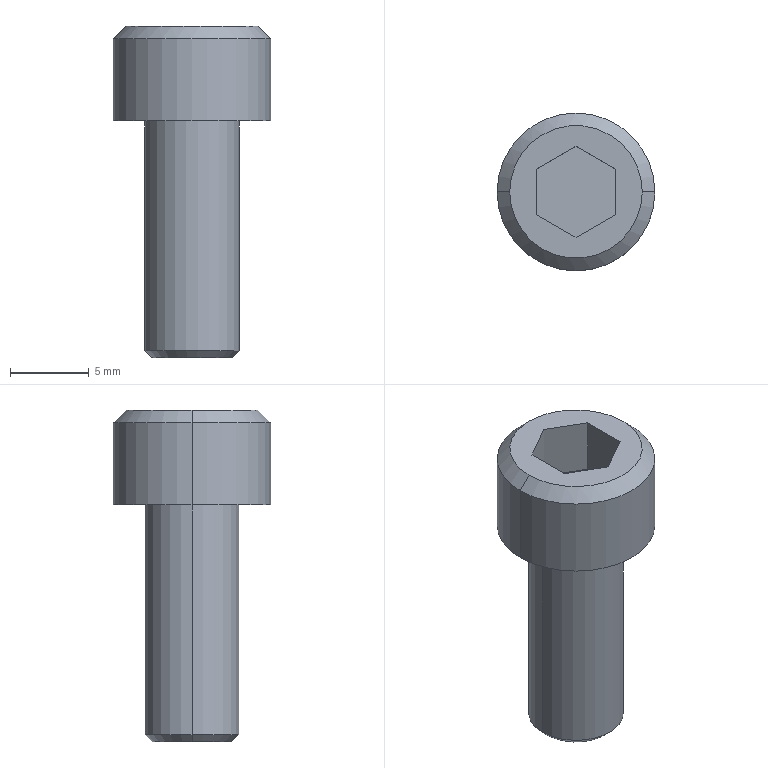Part | Creo | 1 solid | 18 faces | box 10 x 10 x 21 mm | volume 806.082 mm3 | plane 10 | cylinder 4 | cone 4 | commonest cylinder face diameters 6 x2 10 x2
STEP:
#1=CARTESIAN_POINT('',(-255.,152.592,-6.5));
#2=VERTEX_POINT('',#1);
#3=CARTESIAN_POINT('',(-265.,152.592,-6.5));
#4=VERTEX_POINT('',#3);
#5=CARTESIAN_POINT('',(-260.,152.592,-6.5));
#6=DIRECTION('',(0.,0.,-1.));
#7=DIRECTION('',(1.,0.,0.));
#8=AXIS2_PLACEMENT_3D('',#5,#6,#7);
#9=CIRCLE('',#8,5.);
#10=EDGE_CURVE('',#2,#4,#9,.T.);
#11=ORIENTED_EDGE('',*,*,#10,.F.);
#12=CARTESIAN_POINT('',(-260.,152.592,-6.5));
#13=DIRECTION('',(0.,0.,-1.));
#14=DIRECTION('',(-1.,0.,0.));
#15=AXIS2_PLACEMENT_3D('',#12,#13,#14);
#16=CIRCLE('',#15,5.);
#17=EDGE_CURVE('',#4,#2,#16,.T.);
#18=ORIENTED_EDGE('',*,*,#17,.F.);
#19=EDGE_LOOP('',(#11,#18));
#20=FACE_OUTER_BOUND('',#19,.F.);
#21=CARTESIAN_POINT('',(-263.,152.592,-6.5));
#22=VERTEX_POINT('',#21);
#23=CARTESIAN_POINT('',(-257.,152.592,-6.5));
#24=VERTEX_POINT('',#23);
#25=CARTESIAN_POINT('',(-260.,152.592,-6.5));
#26=DIRECTION('',(0.,0.,1.));
#27=DIRECTION('',(-1.,0.,0.));
#28=AXIS2_PLACEMENT_3D('',#25,#26,#27);
#29=CIRCLE('',#28,3.);
#30=EDGE_CURVE('',#22,#24,#29,.T.);
#31=ORIENTED_EDGE('',*,*,#30,.F.);
#32=CARTESIAN_POINT('',(-260.,152.592,-6.5));
#33=DIRECTION('',(0.,0.,1.));
#34=DIRECTION('',(1.,0.,0.));
#35=AXIS2_PLACEMENT_3D('',#32,#33,#34);
#36=CIRCLE('',#35,3.);
#37=EDGE_CURVE('',#24,#22,#36,.T.);
#38=ORIENTED_EDGE('',*,*,#37,.F.);
#39=EDGE_LOOP('',(#31,#38));
#40=FACE_BOUND('',#39,.F.);
#41=CARTESIAN_POINT('',(-260.,152.592,-6.5));
#42=DIRECTION('',(0.,0.,-1.));
#43=DIRECTION('',(-1.,0.,0.));
#44=AXIS2_PLACEMENT_3D('',#41,#42,#43);
#45=PLANE('',#44);
#46=ADVANCED_FACE('',(#20,#40),#45,.T.);
#47=CARTESIAN_POINT('',(-257.,152.592,-21.05));
#48=VERTEX_POINT('',#47);
#49=CARTESIAN_POINT('',(-263.,152.592,-21.05));
#50=VERTEX_POINT('',#49);
#51=CARTESIAN_POINT('',(-260.,152.592,-21.05));
#52=DIRECTION('',(0.,0.,-1.));
#53=DIRECTION('',(1.,0.,0.));
#54=AXIS2_PLACEMENT_3D('',#51,#52,#53);
#55=CIRCLE('',#54,3.);
#56=EDGE_CURVE('',#48,#50,#55,.T.);
#57=ORIENTED_EDGE('',*,*,#56,.T.);
#58=CARTESIAN_POINT('',(-263.,152.592,-6.5));
#59=DIRECTION('',(0.,0.,-1.));
#60=VECTOR('',#59,14.55);
#61=LINE('',#58,#60);
#62=EDGE_CURVE('',#22,#50,#61,.T.);
#63=ORIENTED_EDGE('',*,*,#62,.F.);
#64=ORIENTED_EDGE('',*,*,#30,.T.);
#65=CARTESIAN_POINT('',(-257.,152.592,-6.5));
#66=DIRECTION('',(0.,0.,-1.));
#67=VECTOR('',#66,14.55);
#68=LINE('',#65,#67);
#69=EDGE_CURVE('',#24,#48,#68,.T.);
#70=ORIENTED_EDGE('',*,*,#69,.T.);
#71=EDGE_LOOP('',(#57,#63,#64,#70));
#72=FACE_OUTER_BOUND('',#71,.F.);
#73=CARTESIAN_POINT('',(-260.,152.592,0.5));
#74=DIRECTION('',(0.,0.,-1.));
#75=DIRECTION('',(-1.,0.,0.));
#76=AXIS2_PLACEMENT_3D('',#73,#74,#75);
#77=CYLINDRICAL_SURFACE('',#76,3.);
#78=ADVANCED_FACE('',(#72),#77,.T.);
#79=CARTESIAN_POINT('',(-257.45,152.592,-21.5));
#80=VERTEX_POINT('',#79);
#81=CARTESIAN_POINT('',(-262.55,152.592,-21.5));
#82=VERTEX_POINT('',#81);
#83=CARTESIAN_POINT('',(-260.,152.592,-21.5));
#84=DIRECTION('',(0.,0.,-1.));
#85=DIRECTION('',(1.,0.,0.));
#86=AXIS2_PLACEMENT_3D('',#83,#84,#85);
#87=CIRCLE('',#86,2.55);
#88=EDGE_CURVE('',#80,#82,#87,.T.);
#89=ORIENTED_EDGE('',*,*,#88,.T.);
#90=CARTESIAN_POINT('',(-262.55,152.592,-21.5));
#91=DIRECTION('',(-0.7071,0.,0.7071));
#92=VECTOR('',#91,0.6364);
#93=LINE('',#90,#92);
#94=EDGE_CURVE('',#82,#50,#93,.T.);
#95=ORIENTED_EDGE('',*,*,#94,.T.);
#96=ORIENTED_EDGE('',*,*,#56,.F.);
#97=CARTESIAN_POINT('',(-257.45,152.592,-21.5));
#98=DIRECTION('',(0.7071,0.,0.7071));
#99=VECTOR('',#98,0.6364);
#100=LINE('',#97,#99);
#101=EDGE_CURVE('',#80,#48,#100,.T.);
#102=ORIENTED_EDGE('',*,*,#101,.F.);
#103=EDGE_LOOP('',(#89,#95,#96,#102));
#104=FACE_OUTER_BOUND('',#103,.F.);
#105=CARTESIAN_POINT('',(-260.,152.592,-21.275));
#106=DIRECTION('',(0.,0.,1.));
#107=DIRECTION('',(1.,0.,0.));
#108=AXIS2_PLACEMENT_3D('',#105,#106,#107);
#109=CONICAL_SURFACE('',#108,2.775,45.);
#110=ADVANCED_FACE('',(#104),#109,.T.);
#111=CARTESIAN_POINT('',(-260.,152.592,-21.5));
#112=DIRECTION('',(0.,0.,-1.));
#113=DIRECTION('',(-1.,0.,0.));
#114=AXIS2_PLACEMENT_3D('',#111,#112,#113);
#115=CIRCLE('',#114,2.55);
#116=EDGE_CURVE('',#82,#80,#115,.T.);
#117=ORIENTED_EDGE('',*,*,#116,.F.);
#118=ORIENTED_EDGE('',*,*,#88,.F.);
#119=EDGE_LOOP('',(#117,#118));
#120=FACE_OUTER_BOUND('',#119,.F.);
#121=CARTESIAN_POINT('',(-260.,152.592,-21.5));
#122=DIRECTION('',(0.,0.,-1.));
#123=DIRECTION('',(-1.,0.,0.));
#124=AXIS2_PLACEMENT_3D('',#121,#122,#123);
#125=PLANE('',#124);
#126=ADVANCED_FACE('',(#120),#125,.T.);
#127=ORIENTED_EDGE('',*,*,#116,.T.);
#128=ORIENTED_EDGE('',*,*,#101,.T.);
#129=CARTESIAN_POINT('',(-260.,152.592,-21.05));
#130=DIRECTION('',(0.,0.,-1.));
#131=DIRECTION('',(-1.,0.,0.));
#132=AXIS2_PLACEMENT_3D('',#129,#130,#131);
#133=CIRCLE('',#132,3.);
#134=EDGE_CURVE('',#50,#48,#133,.T.);
#135=ORIENTED_EDGE('',*,*,#134,.F.);
#136=ORIENTED_EDGE('',*,*,#94,.F.);
#137=EDGE_LOOP('',(#127,#128,#135,#136));
#138=FACE_OUTER_BOUND('',#137,.F.);
#139=CARTESIAN_POINT('',(-260.,152.592,-21.275));
#140=DIRECTION('',(0.,0.,1.));
#141=DIRECTION('',(1.,0.,0.));
#142=AXIS2_PLACEMENT_3D('',#139,#140,#141);
#143=CONICAL_SURFACE('',#142,2.775,45.);
#144=ADVANCED_FACE('',(#138),#143,.T.);
#145=ORIENTED_EDGE('',*,*,#134,.T.);
#146=ORIENTED_EDGE('',*,*,#69,.F.);
#147=ORIENTED_EDGE('',*,*,#37,.T.);
#148=ORIENTED_EDGE('',*,*,#62,.T.);
#149=EDGE_LOOP('',(#145,#146,#147,#148));
#150=FACE_OUTER_BOUND('',#149,.F.);
#151=CARTESIAN_POINT('',(-260.,152.592,0.5));
#152=DIRECTION('',(0.,0.,-1.));
#153=DIRECTION('',(-1.,0.,0.));
#154=AXIS2_PLACEMENT_3D('',#151,#152,#153);
#155=CYLINDRICAL_SURFACE('',#154,3.);
#156=ADVANCED_FACE('',(#150),#155,.T.);
#157=CARTESIAN_POINT('',(-265.,152.592,-1.3));
#158=VERTEX_POINT('',#157);
#159=CARTESIAN_POINT('',(-255.,152.592,-1.3));
#160=VERTEX_POINT('',#159);
#161=CARTESIAN_POINT('',(-260.,152.592,-1.3));
#162=DIRECTION('',(0.,0.,1.));
#163=DIRECTION('',(-1.,0.,0.));
#164=AXIS2_PLACEMENT_3D('',#161,#162,#163);
#165=CIRCLE('',#164,5.);
#166=EDGE_CURVE('',#158,#160,#165,.T.);
#167=ORIENTED_EDGE('',*,*,#166,.T.);
#168=CARTESIAN_POINT('',(-255.,152.592,-1.3));
#169=DIRECTION('',(0.,0.,-1.));
#170=VECTOR('',#169,5.2);
#171=LINE('',#168,#170);
#172=EDGE_CURVE('',#160,#2,#171,.T.);
#173=ORIENTED_EDGE('',*,*,#172,.T.);
#174=ORIENTED_EDGE('',*,*,#10,.T.);
#175=CARTESIAN_POINT('',(-265.,152.592,-1.3));
#176=DIRECTION('',(0.,0.,-1.));
#177=VECTOR('',#176,5.2);
#178=LINE('',#175,#177);
#179=EDGE_CURVE('',#158,#4,#178,.T.);
#180=ORIENTED_EDGE('',*,*,#179,.F.);
#181=EDGE_LOOP('',(#167,#173,#174,#180));
#182=FACE_OUTER_BOUND('',#181,.F.);
#183=CARTESIAN_POINT('',(-260.,152.592,0.5));
#184=DIRECTION('',(0.,0.,-1.));
#185=DIRECTION('',(-1.,0.,0.));
#186=AXIS2_PLACEMENT_3D('',#183,#184,#185);
#187=CYLINDRICAL_SURFACE('',#186,5.);
#188=ADVANCED_FACE('',(#182),#187,.T.);
#189=CARTESIAN_POINT('',(-264.2,152.592,-0.5));
#190=VERTEX_POINT('',#189);
#191=CARTESIAN_POINT('',(-255.8,152.592,-0.5));
#192=VERTEX_POINT('',#191);
#193=CARTESIAN_POINT('',(-260.,152.592,-0.5));
#194=DIRECTION('',(0.,0.,1.));
#195=DIRECTION('',(-1.,0.,0.));
#196=AXIS2_PLACEMENT_3D('',#193,#194,#195);
#197=CIRCLE('',#196,4.2);
#198=EDGE_CURVE('',#190,#192,#197,.T.);
#199=ORIENTED_EDGE('',*,*,#198,.T.);
#200=CARTESIAN_POINT('',(-255.8,152.592,-0.5));
#201=DIRECTION('',(0.7071,0.,-0.7071));
#202=VECTOR('',#201,1.131);
#203=LINE('',#200,#202);
#204=EDGE_CURVE('',#192,#160,#203,.T.);
#205=ORIENTED_EDGE('',*,*,#204,.T.);
#206=ORIENTED_EDGE('',*,*,#166,.F.);
#207=CARTESIAN_POINT('',(-264.2,152.592,-0.5));
#208=DIRECTION('',(-0.7071,0.,-0.7071));
#209=VECTOR('',#208,1.131);
#210=LINE('',#207,#209);
#211=EDGE_CURVE('',#190,#158,#210,.T.);
#212=ORIENTED_EDGE('',*,*,#211,.F.);
#213=EDGE_LOOP('',(#199,#205,#206,#212));
#214=FACE_OUTER_BOUND('',#213,.F.);
#215=CARTESIAN_POINT('',(-260.,152.592,-0.9));
#216=DIRECTION('',(0.,0.,-1.));
#217=DIRECTION('',(-1.,0.,0.));
#218=AXIS2_PLACEMENT_3D('',#215,#216,#217);
#219=CONICAL_SURFACE('',#218,4.6,45.);
#220=ADVANCED_FACE('',(#214),#219,.T.);
#221=ORIENTED_EDGE('',*,*,#198,.F.);
#222=CARTESIAN_POINT('',(-260.,152.592,-0.5));
#223=DIRECTION('',(0.,0.,1.));
#224=DIRECTION('',(1.,0.,0.));
#225=AXIS2_PLACEMENT_3D('',#222,#223,#224);
#226=CIRCLE('',#225,4.2);
#227=EDGE_CURVE('',#192,#190,#226,.T.);
#228=ORIENTED_EDGE('',*,*,#227,.F.);
#229=EDGE_LOOP('',(#221,#228));
#230=FACE_OUTER_BOUND('',#229,.F.);
#231=CARTESIAN_POINT('',(-257.5,151.149,-0.5));
#232=VERTEX_POINT('',#231);
#233=CARTESIAN_POINT('',(-260.,149.706,-0.5));
#234=VERTEX_POINT('',#233);
#235=CARTESIAN_POINT('',(-257.5,151.149,-0.5));
#236=DIRECTION('',(-0.866,-0.5,0.));
#237=VECTOR('',#236,2.887);
#238=LINE('',#235,#237);
#239=EDGE_CURVE('',#232,#234,#238,.T.);
#240=ORIENTED_EDGE('',*,*,#239,.F.);
#241=CARTESIAN_POINT('',(-257.5,154.036,-0.5));
#242=VERTEX_POINT('',#241);
#243=CARTESIAN_POINT('',(-257.5,154.036,-0.5));
#244=DIRECTION('',(0.,-1.,0.));
#245=VECTOR('',#244,2.887);
#246=LINE('',#243,#245);
#247=EDGE_CURVE('',#242,#232,#246,.T.);
#248=ORIENTED_EDGE('',*,*,#247,.F.);
#249=CARTESIAN_POINT('',(-260.,155.479,-0.5));
#250=VERTEX_POINT('',#249);
#251=CARTESIAN_POINT('',(-260.,155.479,-0.5));
#252=DIRECTION('',(0.866,-0.5,0.));
#253=VECTOR('',#252,2.887);
#254=LINE('',#251,#253);
#255=EDGE_CURVE('',#250,#242,#254,.T.);
#256=ORIENTED_EDGE('',*,*,#255,.F.);
#257=CARTESIAN_POINT('',(-262.5,154.036,-0.5));
#258=VERTEX_POINT('',#257);
#259=CARTESIAN_POINT('',(-262.5,154.036,-0.5));
#260=DIRECTION('',(0.866,0.5,0.));
#261=VECTOR('',#260,2.887);
#262=LINE('',#259,#261);
#263=EDGE_CURVE('',#258,#250,#262,.T.);
#264=ORIENTED_EDGE('',*,*,#263,.F.);
#265=CARTESIAN_POINT('',(-262.5,151.149,-0.5));
#266=VERTEX_POINT('',#265);
#267=CARTESIAN_POINT('',(-262.5,151.149,-0.5));
#268=DIRECTION('',(0.,1.,0.));
#269=VECTOR('',#268,2.887);
#270=LINE('',#267,#269);
#271=EDGE_CURVE('',#266,#258,#270,.T.);
#272=ORIENTED_EDGE('',*,*,#271,.F.);
#273=CARTESIAN_POINT('',(-260.,149.706,-0.5));
#274=DIRECTION('',(-0.866,0.5,0.));
#275=VECTOR('',#274,2.887);
#276=LINE('',#273,#275);
#277=EDGE_CURVE('',#234,#266,#276,.T.);
#278=ORIENTED_EDGE('',*,*,#277,.F.);
#279=EDGE_LOOP('',(#240,#248,#256,#264,#272,#278));
#280=FACE_BOUND('',#279,.F.);
#281=CARTESIAN_POINT('',(-260.,152.592,-0.5));
#282=DIRECTION('',(0.,0.,-1.));
#283=DIRECTION('',(-1.,0.,0.));
#284=AXIS2_PLACEMENT_3D('',#281,#282,#283);
#285=PLANE('',#284);
#286=ADVANCED_FACE('',(#230,#280),#285,.F.);
#287=ORIENTED_EDGE('',*,*,#227,.T.);
#288=ORIENTED_EDGE('',*,*,#211,.T.);
#289=CARTESIAN_POINT('',(-260.,152.592,-1.3));
#290=DIRECTION('',(0.,0.,1.));
#291=DIRECTION('',(1.,0.,0.));
#292=AXIS2_PLACEMENT_3D('',#289,#290,#291);
#293=CIRCLE('',#292,5.);
#294=EDGE_CURVE('',#160,#158,#293,.T.);
#295=ORIENTED_EDGE('',*,*,#294,.F.);
#296=ORIENTED_EDGE('',*,*,#204,.F.);
#297=EDGE_LOOP('',(#287,#288,#295,#296));
#298=FACE_OUTER_BOUND('',#297,.F.);
#299=CARTESIAN_POINT('',(-260.,152.592,-0.9));
#300=DIRECTION('',(0.,0.,-1.));
#301=DIRECTION('',(-1.,0.,0.));
#302=AXIS2_PLACEMENT_3D('',#299,#300,#301);
#303=CONICAL_SURFACE('',#302,4.6,45.);
#304=ADVANCED_FACE('',(#298),#303,.T.);
#305=ORIENTED_EDGE('',*,*,#294,.T.);
#306=ORIENTED_EDGE('',*,*,#179,.T.);
#307=ORIENTED_EDGE('',*,*,#17,.T.);
#308=ORIENTED_EDGE('',*,*,#172,.F.);
#309=EDGE_LOOP('',(#305,#306,#307,#308));
#310=FACE_OUTER_BOUND('',#309,.F.);
#311=CARTESIAN_POINT('',(-260.,152.592,0.5));
#312=DIRECTION('',(0.,0.,-1.));
#313=DIRECTION('',(-1.,0.,0.));
#314=AXIS2_PLACEMENT_3D('',#311,#312,#313);
#315=CYLINDRICAL_SURFACE('',#314,5.);
#316=ADVANCED_FACE('',(#310),#315,.T.);
#317=ORIENTED_EDGE('',*,*,#239,.T.);
#318=CARTESIAN_POINT('',(-260.,149.706,-4.1));
#319=VERTEX_POINT('',#318);
#320=CARTESIAN_POINT('',(-260.,149.706,-0.5));
#321=DIRECTION('',(0.,0.,-1.));
#322=VECTOR('',#321,3.6);
#323=LINE('',#320,#322);
#324=EDGE_CURVE('',#234,#319,#323,.T.);
#325=ORIENTED_EDGE('',*,*,#324,.T.);
#326=CARTESIAN_POINT('',(-257.5,151.149,-4.1));
#327=VERTEX_POINT('',#326);
#328=CARTESIAN_POINT('',(-260.,149.706,-4.1));
#329=DIRECTION('',(0.866,0.5,0.));
#330=VECTOR('',#329,2.887);
#331=LINE('',#328,#330);
#332=EDGE_CURVE('',#319,#327,#331,.T.);
#333=ORIENTED_EDGE('',*,*,#332,.T.);
#334=CARTESIAN_POINT('',(-257.5,151.149,-0.5));
#335=DIRECTION('',(0.,0.,-1.));
#336=VECTOR('',#335,3.6);
#337=LINE('',#334,#336);
#338=EDGE_CURVE('',#232,#327,#337,.T.);
#339=ORIENTED_EDGE('',*,*,#338,.F.);
#340=EDGE_LOOP('',(#317,#325,#333,#339));
#341=FACE_OUTER_BOUND('',#340,.F.);
#342=CARTESIAN_POINT('',(-260.,149.706,-4.1));
#343=DIRECTION('',(0.5,-0.866,0.));
#344=DIRECTION('',(0.866,0.5,0.));
#345=AXIS2_PLACEMENT_3D('',#342,#343,#344);
#346=PLANE('',#345);
#347=ADVANCED_FACE('',(#341),#346,.F.);
#348=ORIENTED_EDGE('',*,*,#277,.T.);
#349=CARTESIAN_POINT('',(-262.5,151.149,-4.1));
#350=VERTEX_POINT('',#349);
#351=CARTESIAN_POINT('',(-262.5,151.149,-0.5));
#352=DIRECTION('',(0.,0.,-1.));
#353=VECTOR('',#352,3.6);
#354=LINE('',#351,#353);
#355=EDGE_CURVE('',#266,#350,#354,.T.);
#356=ORIENTED_EDGE('',*,*,#355,.T.);
#357=CARTESIAN_POINT('',(-262.5,151.149,-4.1));
#358=DIRECTION('',(0.866,-0.5,0.));
#359=VECTOR('',#358,2.887);
#360=LINE('',#357,#359);
#361=EDGE_CURVE('',#350,#319,#360,.T.);
#362=ORIENTED_EDGE('',*,*,#361,.T.);
#363=ORIENTED_EDGE('',*,*,#324,.F.);
#364=EDGE_LOOP('',(#348,#356,#362,#363));
#365=FACE_OUTER_BOUND('',#364,.F.);
#366=CARTESIAN_POINT('',(-262.5,151.149,-4.1));
#367=DIRECTION('',(-0.5,-0.866,0.));
#368=DIRECTION('',(0.866,-0.5,0.));
#369=AXIS2_PLACEMENT_3D('',#366,#367,#368);
#370=PLANE('',#369);
#371=ADVANCED_FACE('',(#365),#370,.F.);
#372=ORIENTED_EDGE('',*,*,#271,.T.);
#373=CARTESIAN_POINT('',(-262.5,154.036,-4.1));
#374=VERTEX_POINT('',#373);
#375=CARTESIAN_POINT('',(-262.5,154.036,-0.5));
#376=DIRECTION('',(0.,0.,-1.));
#377=VECTOR('',#376,3.6);
#378=LINE('',#375,#377);
#379=EDGE_CURVE('',#258,#374,#378,.T.);
#380=ORIENTED_EDGE('',*,*,#379,.T.);
#381=CARTESIAN_POINT('',(-262.5,151.149,-4.1));
#382=DIRECTION('',(0.,1.,0.));
#383=VECTOR('',#382,2.887);
#384=LINE('',#381,#383);
#385=EDGE_CURVE('',#350,#374,#384,.T.);
#386=ORIENTED_EDGE('',*,*,#385,.F.);
#387=ORIENTED_EDGE('',*,*,#355,.F.);
#388=EDGE_LOOP('',(#372,#380,#386,#387));
#389=FACE_OUTER_BOUND('',#388,.F.);
#390=CARTESIAN_POINT('',(-262.5,154.036,-4.1));
#391=DIRECTION('',(-1.,0.,0.));
#392=DIRECTION('',(0.,0.,1.));
#393=AXIS2_PLACEMENT_3D('',#390,#391,#392);
#394=PLANE('',#393);
#395=ADVANCED_FACE('',(#389),#394,.F.);
#396=ORIENTED_EDGE('',*,*,#263,.T.);
#397=CARTESIAN_POINT('',(-260.,155.479,-4.1));
#398=VERTEX_POINT('',#397);
#399=CARTESIAN_POINT('',(-260.,155.479,-0.5));
#400=DIRECTION('',(0.,0.,-1.));
#401=VECTOR('',#400,3.6);
#402=LINE('',#399,#401);
#403=EDGE_CURVE('',#250,#398,#402,.T.);
#404=ORIENTED_EDGE('',*,*,#403,.T.);
#405=CARTESIAN_POINT('',(-260.,155.479,-4.1));
#406=DIRECTION('',(-0.866,-0.5,0.));
#407=VECTOR('',#406,2.887);
#408=LINE('',#405,#407);
#409=EDGE_CURVE('',#398,#374,#408,.T.);
#410=ORIENTED_EDGE('',*,*,#409,.T.);
#411=ORIENTED_EDGE('',*,*,#379,.F.);
#412=EDGE_LOOP('',(#396,#404,#410,#411));
#413=FACE_OUTER_BOUND('',#412,.F.);
#414=CARTESIAN_POINT('',(-260.,155.479,-4.1));
#415=DIRECTION('',(-0.5,0.866,0.));
#416=DIRECTION('',(-0.866,-0.5,0.));
#417=AXIS2_PLACEMENT_3D('',#414,#415,#416);
#418=PLANE('',#417);
#419=ADVANCED_FACE('',(#413),#418,.F.);
#420=ORIENTED_EDGE('',*,*,#255,.T.);
#421=CARTESIAN_POINT('',(-257.5,154.036,-4.1));
#422=VERTEX_POINT('',#421);
#423=CARTESIAN_POINT('',(-257.5,154.036,-0.5));
#424=DIRECTION('',(0.,0.,-1.));
#425=VECTOR('',#424,3.6);
#426=LINE('',#423,#425);
#427=EDGE_CURVE('',#242,#422,#426,.T.);
#428=ORIENTED_EDGE('',*,*,#427,.T.);
#429=CARTESIAN_POINT('',(-257.5,154.036,-4.1));
#430=DIRECTION('',(-0.866,0.5,0.));
#431=VECTOR('',#430,2.887);
#432=LINE('',#429,#431);
#433=EDGE_CURVE('',#422,#398,#432,.T.);
#434=ORIENTED_EDGE('',*,*,#433,.T.);
#435=ORIENTED_EDGE('',*,*,#403,.F.);
#436=EDGE_LOOP('',(#420,#428,#434,#435));
#437=FACE_OUTER_BOUND('',#436,.F.);
#438=CARTESIAN_POINT('',(-257.5,154.036,-4.1));
#439=DIRECTION('',(0.5,0.866,0.));
#440=DIRECTION('',(-0.866,0.5,0.));
#441=AXIS2_PLACEMENT_3D('',#438,#439,#440);
#442=PLANE('',#441);
#443=ADVANCED_FACE('',(#437),#442,.F.);
#444=ORIENTED_EDGE('',*,*,#247,.T.);
#445=ORIENTED_EDGE('',*,*,#338,.T.);
#446=CARTESIAN_POINT('',(-257.5,154.036,-4.1));
#447=DIRECTION('',(0.,-1.,0.));
#448=VECTOR('',#447,2.887);
#449=LINE('',#446,#448);
#450=EDGE_CURVE('',#422,#327,#449,.T.);
#451=ORIENTED_EDGE('',*,*,#450,.F.);
#452=ORIENTED_EDGE('',*,*,#427,.F.);
#453=EDGE_LOOP('',(#444,#445,#451,#452));
#454=FACE_OUTER_BOUND('',#453,.F.);
#455=CARTESIAN_POINT('',(-257.5,151.149,-4.1));
#456=DIRECTION('',(1.,0.,0.));
#457=DIRECTION('',(0.,0.,-1.));
#458=AXIS2_PLACEMENT_3D('',#455,#456,#457);
#459=PLANE('',#458);
#460=ADVANCED_FACE('',(#454),#459,.F.);
#461=ORIENTED_EDGE('',*,*,#361,.F.);
#462=ORIENTED_EDGE('',*,*,#385,.T.);
#463=ORIENTED_EDGE('',*,*,#409,.F.);
#464=ORIENTED_EDGE('',*,*,#433,.F.);
#465=ORIENTED_EDGE('',*,*,#450,.T.);
#466=ORIENTED_EDGE('',*,*,#332,.F.);
#467=EDGE_LOOP('',(#461,#462,#463,#464,#465,#466));
#468=FACE_OUTER_BOUND('',#467,.F.);
#469=CARTESIAN_POINT('',(-257.5,148.262,-4.1));
#470=DIRECTION('',(0.,0.,1.));
#471=DIRECTION('',(1.,0.,0.));
#472=AXIS2_PLACEMENT_3D('',#469,#470,#471);
#473=PLANE('',#472);
#474=ADVANCED_FACE('',(#468),#473,.T.);
#475=CLOSED_SHELL('',(#46,#78,#110,#126,#144,#156,#188,#220,#286,#304,#316,#347,#371,#395,#419,#443,#460,#474));
#476=MANIFOLD_SOLID_BREP('',#475);
#477=(LENGTH_UNIT()NAMED_UNIT(*)SI_UNIT(.MILLI.,.METRE.));
#478=UNCERTAINTY_MEASURE_WITH_UNIT(LENGTH_MEASURE(0.002532),#477,'','');
#479=(NAMED_UNIT(*)PLANE_ANGLE_UNIT()SI_UNIT($,.RADIAN.));
#480=PLANE_ANGLE_MEASURE_WITH_UNIT(PLANE_ANGLE_MEASURE(0.01745),#479);
#481=(CONVERSION_BASED_UNIT('DEGREE',#480)NAMED_UNIT(*)PLANE_ANGLE_UNIT());
#482=(NAMED_UNIT(*)SI_UNIT($,.STERADIAN.)SOLID_ANGLE_UNIT());
#483=(GEOMETRIC_REPRESENTATION_CONTEXT(3)GLOBAL_UNCERTAINTY_ASSIGNED_CONTEXT((#478))GLOBAL_UNIT_ASSIGNED_CONTEXT((#477,#481,#482))REPRESENTATION_CONTEXT('',''));
#484=ADVANCED_BREP_SHAPE_REPRESENTATION('',(#476),#483);